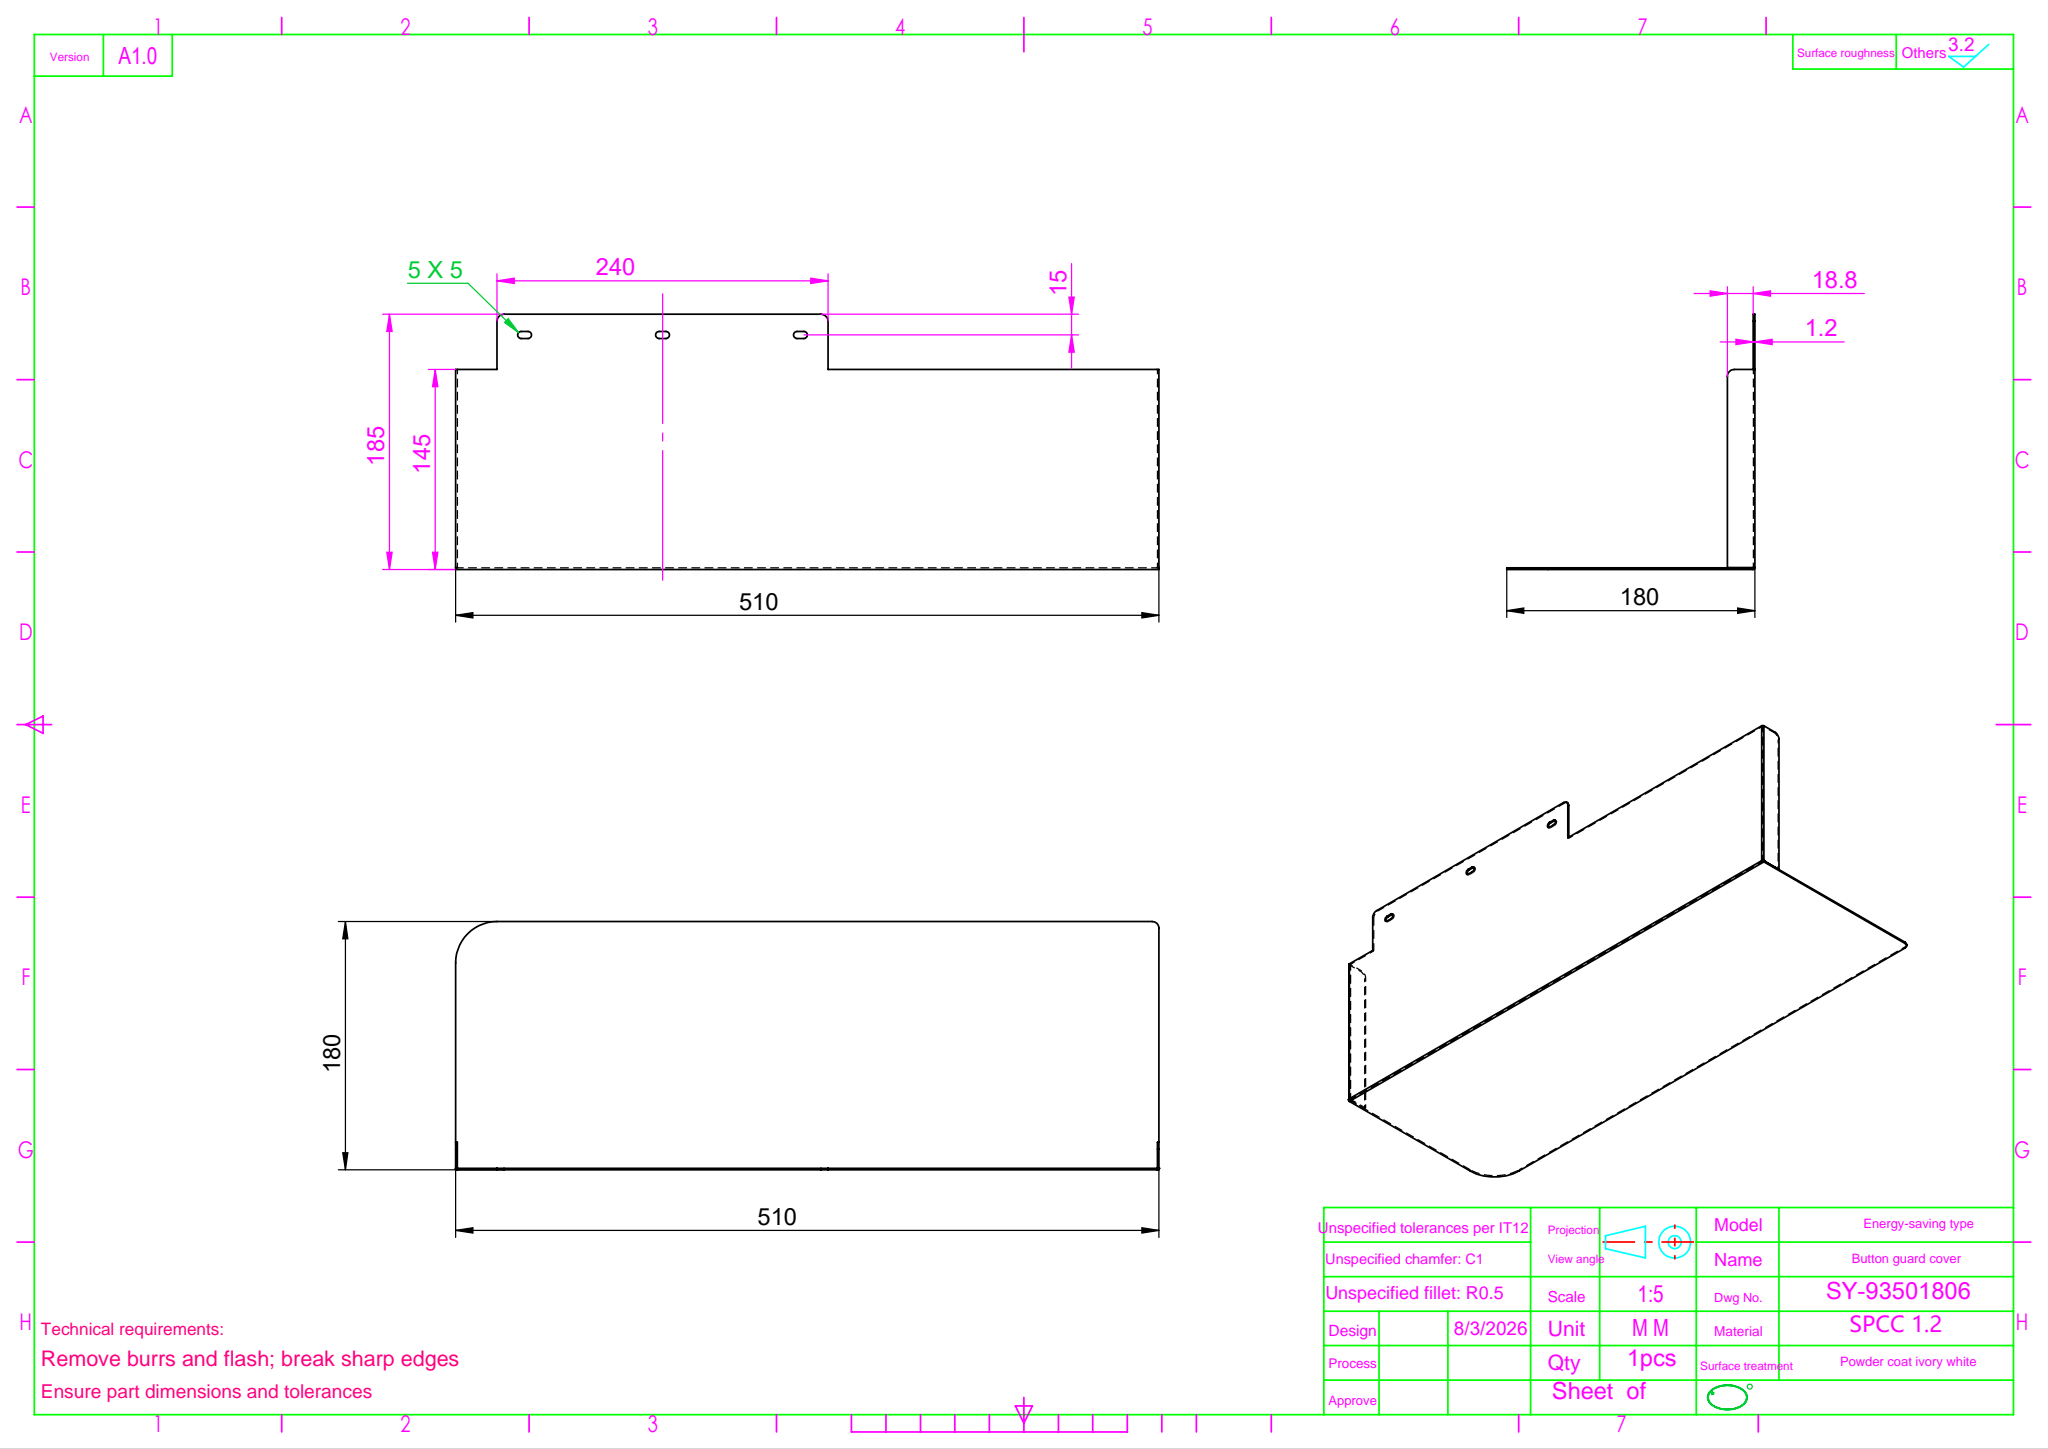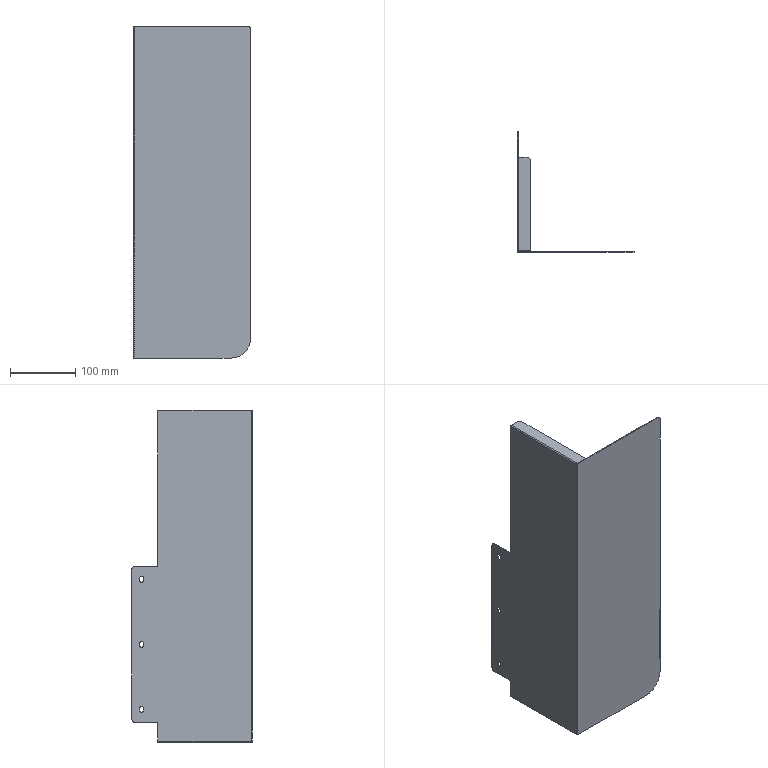Part | SolidWorks | features Fillet 2, ICE 2, EdgeFlange 1, FlatPattern 1, LPattern 1, MoveFace 1, SMBaseFlange 1, SheetMetal 1 | 1 solid | 53 faces | box 180 x 185 x 510 mm | volume 215412 mm3 | plane 32 | cylinder 21 | commonest cylinder face diameters 5 x9 10 x5 0.4 x3 2.8 x3 60 x1